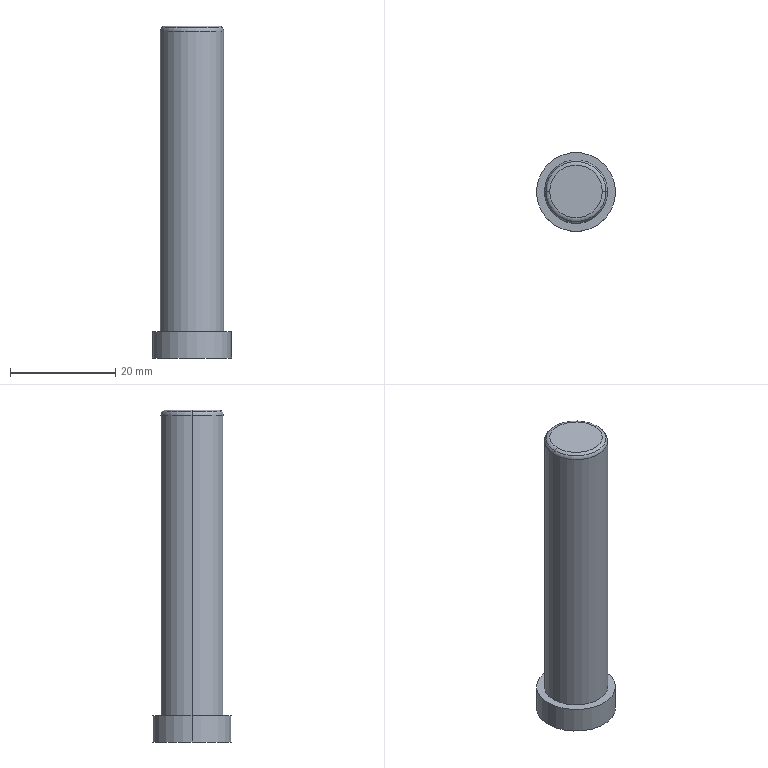Part | STEP file | 1_id1318_x_t | 1 solid | 11 faces | box 15 x 15 x 63 mm | volume 7435 mm3 | cylinder 4 | torus 4 | plane 3 | commonest cylinder face diameters 12 x2 15 x2
STEP:
#1=CARTESIAN_POINT('',(0.,0.,0.));
#2=DIRECTION('',(0.,0.,1.));
#3=DIRECTION('',(1.,0.,0.));
#4=AXIS2_PLACEMENT_3D('',#1,#2,#3);
#5=CARTESIAN_POINT('',(86.275,141.9,-58.));
#6=VERTEX_POINT('',#5);
#7=CARTESIAN_POINT('',(86.275,141.9,-1.));
#8=VERTEX_POINT('',#7);
#9=CARTESIAN_POINT('',(86.275,141.9,-58.));
#10=DIRECTION('',(0.,0.,1.));
#11=VECTOR('',#10,1.);
#12=LINE('',#9,#11);
#13=CARTESIAN_POINT('',(92.275,141.9,-50.));
#14=DIRECTION('',(0.,0.,1.));
#15=DIRECTION('',(1.,0.,0.));
#16=AXIS2_PLACEMENT_3D('',#13,#14,#15);
#17=CYLINDRICAL_SURFACE('',#16,6.);
#18=CARTESIAN_POINT('',(3.142,-8.));
#19=DIRECTION('',(0.,1.));
#20=VECTOR('',#19,1.);
#21=LINE('',#18,#20);
#22=(GEOMETRIC_REPRESENTATION_CONTEXT(2)PARAMETRIC_REPRESENTATION_CONTEXT()REPRESENTATION_CONTEXT('',''));
#23=DEFINITIONAL_REPRESENTATION('',(#21),#22);
#24=PCURVE('',#17,#23);
#25=CARTESIAN_POINT('',(92.275,141.9,-50.));
#26=DIRECTION('',(0.,0.,1.));
#27=DIRECTION('',(1.,0.,0.));
#28=AXIS2_PLACEMENT_3D('',#25,#26,#27);
#29=CYLINDRICAL_SURFACE('',#28,6.);
#30=CARTESIAN_POINT('',(3.142,-8.));
#31=DIRECTION('',(0.,1.));
#32=VECTOR('',#31,1.);
#33=LINE('',#30,#32);
#34=(GEOMETRIC_REPRESENTATION_CONTEXT(2)PARAMETRIC_REPRESENTATION_CONTEXT()REPRESENTATION_CONTEXT('',''));
#35=DEFINITIONAL_REPRESENTATION('',(#33),#34);
#36=PCURVE('',#29,#35);
#37=SURFACE_CURVE('',#12,(#24,#36),.PCURVE_S1.);
#38=EDGE_CURVE('',#6,#8,#37,.T.);
#39=ORIENTED_EDGE('',*,*,#38,.F.);
#40=CARTESIAN_POINT('',(98.275,141.9,-58.));
#41=VERTEX_POINT('',#40);
#42=CARTESIAN_POINT('',(92.275,141.9,-58.));
#43=DIRECTION('',(0.,0.,-1.));
#44=DIRECTION('',(1.,0.,0.));
#45=AXIS2_PLACEMENT_3D('',#42,#43,#44);
#46=CIRCLE('',#45,6.);
#47=CARTESIAN_POINT('',(6.283,-8.));
#48=DIRECTION('',(-1.,0.));
#49=VECTOR('',#48,1.);
#50=LINE('',#47,#49);
#51=(GEOMETRIC_REPRESENTATION_CONTEXT(2)PARAMETRIC_REPRESENTATION_CONTEXT()REPRESENTATION_CONTEXT('',''));
#52=DEFINITIONAL_REPRESENTATION('',(#50),#51);
#53=PCURVE('',#17,#52);
#54=CARTESIAN_POINT('',(92.275,141.9,-58.));
#55=DIRECTION('',(0.,0.,-1.));
#56=DIRECTION('',(-1.,0.,0.));
#57=AXIS2_PLACEMENT_3D('',#54,#55,#56);
#58=PLANE('',#57);
#59=CARTESIAN_POINT('',(0.,0.));
#60=DIRECTION('',(-1.,0.));
#61=AXIS2_PLACEMENT_2D('',#59,#60);
#62=CIRCLE('',#61,6.);
#63=(GEOMETRIC_REPRESENTATION_CONTEXT(2)PARAMETRIC_REPRESENTATION_CONTEXT()REPRESENTATION_CONTEXT('',''));
#64=DEFINITIONAL_REPRESENTATION('',(#62),#63);
#65=PCURVE('',#58,#64);
#66=SURFACE_CURVE('',#46,(#53,#65),.PCURVE_S1.);
#67=EDGE_CURVE('',#41,#6,#66,.T.);
#68=ORIENTED_EDGE('',*,*,#67,.F.);
#69=CARTESIAN_POINT('',(98.275,141.9,-1.));
#70=VERTEX_POINT('',#69);
#71=CARTESIAN_POINT('',(98.275,141.9,-58.));
#72=DIRECTION('',(0.,0.,-1.));
#73=VECTOR('',#72,1.);
#74=LINE('',#71,#73);
#75=CARTESIAN_POINT('',(6.283,-8.));
#76=DIRECTION('',(0.,-1.));
#77=VECTOR('',#76,1.);
#78=LINE('',#75,#77);
#79=(GEOMETRIC_REPRESENTATION_CONTEXT(2)PARAMETRIC_REPRESENTATION_CONTEXT()REPRESENTATION_CONTEXT('',''));
#80=DEFINITIONAL_REPRESENTATION('',(#78),#79);
#81=PCURVE('',#17,#80);
#82=CARTESIAN_POINT('',(0.,-8.));
#83=DIRECTION('',(0.,-1.));
#84=VECTOR('',#83,1.);
#85=LINE('',#82,#84);
#86=(GEOMETRIC_REPRESENTATION_CONTEXT(2)PARAMETRIC_REPRESENTATION_CONTEXT()REPRESENTATION_CONTEXT('',''));
#87=DEFINITIONAL_REPRESENTATION('',(#85),#86);
#88=PCURVE('',#29,#87);
#89=SURFACE_CURVE('',#74,(#81,#88),.PCURVE_S1.);
#90=EDGE_CURVE('',#70,#41,#89,.T.);
#91=ORIENTED_EDGE('',*,*,#90,.F.);
#92=CARTESIAN_POINT('',(92.275,141.9,-1.));
#93=DIRECTION('',(0.,0.,1.));
#94=DIRECTION('',(-1.,0.,0.));
#95=AXIS2_PLACEMENT_3D('',#92,#93,#94);
#96=CIRCLE('',#95,6.);
#97=CARTESIAN_POINT('',(3.142,49.));
#98=DIRECTION('',(1.,0.));
#99=VECTOR('',#98,1.);
#100=LINE('',#97,#99);
#101=(GEOMETRIC_REPRESENTATION_CONTEXT(2)PARAMETRIC_REPRESENTATION_CONTEXT()REPRESENTATION_CONTEXT('',''));
#102=DEFINITIONAL_REPRESENTATION('',(#100),#101);
#103=PCURVE('',#17,#102);
#104=CARTESIAN_POINT('',(92.275,141.9,-1.));
#105=DIRECTION('',(0.,0.,1.));
#106=DIRECTION('',(1.,0.,0.));
#107=AXIS2_PLACEMENT_3D('',#104,#105,#106);
#108=TOROIDAL_SURFACE('',#107,5.,1.);
#109=CARTESIAN_POINT('',(3.142,0.));
#110=DIRECTION('',(1.,0.));
#111=VECTOR('',#110,1.);
#112=LINE('',#109,#111);
#113=(GEOMETRIC_REPRESENTATION_CONTEXT(2)PARAMETRIC_REPRESENTATION_CONTEXT()REPRESENTATION_CONTEXT('',''));
#114=DEFINITIONAL_REPRESENTATION('',(#112),#113);
#115=PCURVE('',#108,#114);
#116=SURFACE_CURVE('',#96,(#103,#115),.PCURVE_S1.);
#117=EDGE_CURVE('',#8,#70,#116,.T.);
#118=ORIENTED_EDGE('',*,*,#117,.F.);
#119=EDGE_LOOP('',(#39,#68,#91,#118));
#120=FACE_BOUND('',#119,.T.);
#121=ADVANCED_FACE('',(#120),#17,.T.);
#122=CARTESIAN_POINT('',(97.982,141.9,-0.2929));
#123=VERTEX_POINT('',#122);
#124=CARTESIAN_POINT('',(97.275,141.9,-1.));
#125=DIRECTION('',(0.,1.,0.));
#126=DIRECTION('',(1.,0.,0.));
#127=AXIS2_PLACEMENT_3D('',#124,#125,#126);
#128=CIRCLE('',#127,1.);
#129=CARTESIAN_POINT('',(6.283,6.283));
#130=DIRECTION('',(0.,-1.));
#131=VECTOR('',#130,1.);
#132=LINE('',#129,#131);
#133=(GEOMETRIC_REPRESENTATION_CONTEXT(2)PARAMETRIC_REPRESENTATION_CONTEXT()REPRESENTATION_CONTEXT('',''));
#134=DEFINITIONAL_REPRESENTATION('',(#132),#133);
#135=PCURVE('',#108,#134);
#136=CARTESIAN_POINT('',(92.275,141.9,-1.));
#137=DIRECTION('',(0.,0.,1.));
#138=DIRECTION('',(1.,0.,0.));
#139=AXIS2_PLACEMENT_3D('',#136,#137,#138);
#140=TOROIDAL_SURFACE('',#139,5.,1.);
#141=CARTESIAN_POINT('',(0.,6.283));
#142=DIRECTION('',(0.,-1.));
#143=VECTOR('',#142,1.);
#144=LINE('',#141,#143);
#145=(GEOMETRIC_REPRESENTATION_CONTEXT(2)PARAMETRIC_REPRESENTATION_CONTEXT()REPRESENTATION_CONTEXT('',''));
#146=DEFINITIONAL_REPRESENTATION('',(#144),#145);
#147=PCURVE('',#140,#146);
#148=SURFACE_CURVE('',#128,(#135,#147),.PCURVE_S1.);
#149=EDGE_CURVE('',#123,#70,#148,.T.);
#150=ORIENTED_EDGE('',*,*,#149,.F.);
#151=CARTESIAN_POINT('',(86.568,141.9,-0.2929));
#152=VERTEX_POINT('',#151);
#153=CARTESIAN_POINT('',(92.275,141.9,-0.2929));
#154=DIRECTION('',(0.,0.,1.));
#155=DIRECTION('',(-1.,0.,0.));
#156=AXIS2_PLACEMENT_3D('',#153,#154,#155);
#157=CIRCLE('',#156,5.707);
#158=CARTESIAN_POINT('',(3.142,0.7854));
#159=DIRECTION('',(1.,0.));
#160=VECTOR('',#159,1.);
#161=LINE('',#158,#160);
#162=(GEOMETRIC_REPRESENTATION_CONTEXT(2)PARAMETRIC_REPRESENTATION_CONTEXT()REPRESENTATION_CONTEXT('',''));
#163=DEFINITIONAL_REPRESENTATION('',(#161),#162);
#164=PCURVE('',#108,#163);
#165=CARTESIAN_POINT('',(92.275,141.9,-1.));
#166=DIRECTION('',(0.,0.,1.));
#167=DIRECTION('',(1.,0.,0.));
#168=AXIS2_PLACEMENT_3D('',#165,#166,#167);
#169=TOROIDAL_SURFACE('',#168,5.,1.);
#170=CARTESIAN_POINT('',(3.142,0.7854));
#171=DIRECTION('',(1.,0.));
#172=VECTOR('',#171,1.);
#173=LINE('',#170,#172);
#174=(GEOMETRIC_REPRESENTATION_CONTEXT(2)PARAMETRIC_REPRESENTATION_CONTEXT()REPRESENTATION_CONTEXT('',''));
#175=DEFINITIONAL_REPRESENTATION('',(#173),#174);
#176=PCURVE('',#169,#175);
#177=SURFACE_CURVE('',#157,(#164,#176),.PCURVE_S1.);
#178=EDGE_CURVE('',#152,#123,#177,.T.);
#179=ORIENTED_EDGE('',*,*,#178,.F.);
#180=CARTESIAN_POINT('',(87.275,141.9,-1.));
#181=DIRECTION('',(0.,1.,0.));
#182=DIRECTION('',(-1.,0.,0.));
#183=AXIS2_PLACEMENT_3D('',#180,#181,#182);
#184=CIRCLE('',#183,1.);
#185=CARTESIAN_POINT('',(3.142,0.));
#186=DIRECTION('',(0.,1.));
#187=VECTOR('',#186,1.);
#188=LINE('',#185,#187);
#189=(GEOMETRIC_REPRESENTATION_CONTEXT(2)PARAMETRIC_REPRESENTATION_CONTEXT()REPRESENTATION_CONTEXT('',''));
#190=DEFINITIONAL_REPRESENTATION('',(#188),#189);
#191=PCURVE('',#108,#190);
#192=CARTESIAN_POINT('',(3.142,0.));
#193=DIRECTION('',(0.,1.));
#194=VECTOR('',#193,1.);
#195=LINE('',#192,#194);
#196=(GEOMETRIC_REPRESENTATION_CONTEXT(2)PARAMETRIC_REPRESENTATION_CONTEXT()REPRESENTATION_CONTEXT('',''));
#197=DEFINITIONAL_REPRESENTATION('',(#195),#196);
#198=PCURVE('',#140,#197);
#199=SURFACE_CURVE('',#184,(#191,#198),.PCURVE_S1.);
#200=EDGE_CURVE('',#8,#152,#199,.T.);
#201=ORIENTED_EDGE('',*,*,#200,.F.);
#202=ORIENTED_EDGE('',*,*,#117,.T.);
#203=EDGE_LOOP('',(#150,#179,#201,#202));
#204=FACE_BOUND('',#203,.T.);
#205=ADVANCED_FACE('',(#204),#108,.T.);
#206=ORIENTED_EDGE('',*,*,#200,.T.);
#207=CARTESIAN_POINT('',(92.275,141.9,-0.2929));
#208=DIRECTION('',(0.,0.,1.));
#209=DIRECTION('',(1.,0.,0.));
#210=AXIS2_PLACEMENT_3D('',#207,#208,#209);
#211=CIRCLE('',#210,5.707);
#212=CARTESIAN_POINT('',(0.,0.7854));
#213=DIRECTION('',(1.,0.));
#214=VECTOR('',#213,1.);
#215=LINE('',#212,#214);
#216=(GEOMETRIC_REPRESENTATION_CONTEXT(2)PARAMETRIC_REPRESENTATION_CONTEXT()REPRESENTATION_CONTEXT('',''));
#217=DEFINITIONAL_REPRESENTATION('',(#215),#216);
#218=PCURVE('',#140,#217);
#219=CARTESIAN_POINT('',(92.275,141.9,-1.));
#220=DIRECTION('',(0.,0.,1.));
#221=DIRECTION('',(1.,0.,0.));
#222=AXIS2_PLACEMENT_3D('',#219,#220,#221);
#223=TOROIDAL_SURFACE('',#222,5.,1.);
#224=CARTESIAN_POINT('',(0.,0.7854));
#225=DIRECTION('',(1.,0.));
#226=VECTOR('',#225,1.);
#227=LINE('',#224,#226);
#228=(GEOMETRIC_REPRESENTATION_CONTEXT(2)PARAMETRIC_REPRESENTATION_CONTEXT()REPRESENTATION_CONTEXT('',''));
#229=DEFINITIONAL_REPRESENTATION('',(#227),#228);
#230=PCURVE('',#223,#229);
#231=SURFACE_CURVE('',#211,(#218,#230),.PCURVE_S1.);
#232=EDGE_CURVE('',#123,#152,#231,.T.);
#233=ORIENTED_EDGE('',*,*,#232,.F.);
#234=ORIENTED_EDGE('',*,*,#149,.T.);
#235=CARTESIAN_POINT('',(92.275,141.9,-1.));
#236=DIRECTION('',(0.,0.,1.));
#237=DIRECTION('',(1.,0.,0.));
#238=AXIS2_PLACEMENT_3D('',#235,#236,#237);
#239=CIRCLE('',#238,6.);
#240=CARTESIAN_POINT('',(0.,0.));
#241=DIRECTION('',(1.,0.));
#242=VECTOR('',#241,1.);
#243=LINE('',#240,#242);
#244=(GEOMETRIC_REPRESENTATION_CONTEXT(2)PARAMETRIC_REPRESENTATION_CONTEXT()REPRESENTATION_CONTEXT('',''));
#245=DEFINITIONAL_REPRESENTATION('',(#243),#244);
#246=PCURVE('',#140,#245);
#247=CARTESIAN_POINT('',(0.,49.));
#248=DIRECTION('',(1.,0.));
#249=VECTOR('',#248,1.);
#250=LINE('',#247,#249);
#251=(GEOMETRIC_REPRESENTATION_CONTEXT(2)PARAMETRIC_REPRESENTATION_CONTEXT()REPRESENTATION_CONTEXT('',''));
#252=DEFINITIONAL_REPRESENTATION('',(#250),#251);
#253=PCURVE('',#29,#252);
#254=SURFACE_CURVE('',#239,(#246,#253),.PCURVE_S1.);
#255=EDGE_CURVE('',#70,#8,#254,.T.);
#256=ORIENTED_EDGE('',*,*,#255,.T.);
#257=EDGE_LOOP('',(#206,#233,#234,#256));
#258=FACE_BOUND('',#257,.T.);
#259=ADVANCED_FACE('',(#258),#140,.T.);
#260=ORIENTED_EDGE('',*,*,#90,.T.);
#261=CARTESIAN_POINT('',(92.275,141.9,-58.));
#262=DIRECTION('',(0.,0.,-1.));
#263=DIRECTION('',(-1.,0.,0.));
#264=AXIS2_PLACEMENT_3D('',#261,#262,#263);
#265=CIRCLE('',#264,6.);
#266=CARTESIAN_POINT('',(3.142,-8.));
#267=DIRECTION('',(-1.,0.));
#268=VECTOR('',#267,1.);
#269=LINE('',#266,#268);
#270=(GEOMETRIC_REPRESENTATION_CONTEXT(2)PARAMETRIC_REPRESENTATION_CONTEXT()REPRESENTATION_CONTEXT('',''));
#271=DEFINITIONAL_REPRESENTATION('',(#269),#270);
#272=PCURVE('',#29,#271);
#273=CARTESIAN_POINT('',(0.,0.));
#274=DIRECTION('',(1.,0.));
#275=AXIS2_PLACEMENT_2D('',#273,#274);
#276=CIRCLE('',#275,6.);
#277=(GEOMETRIC_REPRESENTATION_CONTEXT(2)PARAMETRIC_REPRESENTATION_CONTEXT()REPRESENTATION_CONTEXT('',''));
#278=DEFINITIONAL_REPRESENTATION('',(#276),#277);
#279=PCURVE('',#58,#278);
#280=SURFACE_CURVE('',#265,(#272,#279),.PCURVE_S1.);
#281=EDGE_CURVE('',#6,#41,#280,.T.);
#282=ORIENTED_EDGE('',*,*,#281,.F.);
#283=ORIENTED_EDGE('',*,*,#38,.T.);
#284=ORIENTED_EDGE('',*,*,#255,.F.);
#285=EDGE_LOOP('',(#260,#282,#283,#284));
#286=FACE_BOUND('',#285,.T.);
#287=ADVANCED_FACE('',(#286),#29,.T.);
#288=CARTESIAN_POINT('',(84.775,141.9,-58.));
#289=VERTEX_POINT('',#288);
#290=CARTESIAN_POINT('',(99.775,141.9,-58.));
#291=VERTEX_POINT('',#290);
#292=CARTESIAN_POINT('',(92.275,141.9,-58.));
#293=DIRECTION('',(0.,0.,1.));
#294=DIRECTION('',(-1.,0.,0.));
#295=AXIS2_PLACEMENT_3D('',#292,#293,#294);
#296=CIRCLE('',#295,7.5);
#297=CARTESIAN_POINT('',(7.5,0.));
#298=CARTESIAN_POINT('',(7.5,-12.99));
#299=CARTESIAN_POINT('',(-3.75,-6.495));
#300=CARTESIAN_POINT('',(-15.,0.));
#301=CARTESIAN_POINT('',(-3.75,6.495));
#302=CARTESIAN_POINT('',(7.5,12.99));
#303=CARTESIAN_POINT('',(7.5,0.));
#304=(BOUNDED_CURVE()B_SPLINE_CURVE(2,(#297,#298,#299,#300,#301,#302,#303),.UNSPECIFIED.,.T.,.F.)B_SPLINE_CURVE_WITH_KNOTS((1,2,2,2,2,1),(-2.094,0.,2.094,4.189,6.283,8.378),.UNSPECIFIED.)CURVE()GEOMETRIC_REPRESENTATION_ITEM()RATIONAL_B_SPLINE_CURVE((1.,0.5,1.,0.5,1.,0.5,1.))REPRESENTATION_ITEM(''));
#305=(GEOMETRIC_REPRESENTATION_CONTEXT(2)PARAMETRIC_REPRESENTATION_CONTEXT()REPRESENTATION_CONTEXT('',''));
#306=DEFINITIONAL_REPRESENTATION('',(#304),#305);
#307=PCURVE('',#58,#306);
#308=CARTESIAN_POINT('',(92.275,141.9,-58.));
#309=DIRECTION('',(0.,0.,-1.));
#310=DIRECTION('',(-1.,0.,0.));
#311=AXIS2_PLACEMENT_3D('',#308,#309,#310);
#312=CYLINDRICAL_SURFACE('',#311,7.5);
#313=CARTESIAN_POINT('',(6.283,0.));
#314=DIRECTION('',(-1.,0.));
#315=VECTOR('',#314,1.);
#316=LINE('',#313,#315);
#317=(GEOMETRIC_REPRESENTATION_CONTEXT(2)PARAMETRIC_REPRESENTATION_CONTEXT()REPRESENTATION_CONTEXT('',''));
#318=DEFINITIONAL_REPRESENTATION('',(#316),#317);
#319=PCURVE('',#312,#318);
#320=SURFACE_CURVE('',#296,(#307,#319),.PCURVE_S1.);
#321=EDGE_CURVE('',#289,#291,#320,.T.);
#322=ORIENTED_EDGE('',*,*,#321,.T.);
#323=CARTESIAN_POINT('',(92.275,141.9,-58.));
#324=DIRECTION('',(0.,0.,1.));
#325=DIRECTION('',(1.,0.,0.));
#326=AXIS2_PLACEMENT_3D('',#323,#324,#325);
#327=CIRCLE('',#326,7.5);
#328=CARTESIAN_POINT('',(-7.5,0.));
#329=CARTESIAN_POINT('',(-7.5,12.99));
#330=CARTESIAN_POINT('',(3.75,6.495));
#331=CARTESIAN_POINT('',(15.,0.));
#332=CARTESIAN_POINT('',(3.75,-6.495));
#333=CARTESIAN_POINT('',(-7.5,-12.99));
#334=CARTESIAN_POINT('',(-7.5,0.));
#335=(BOUNDED_CURVE()B_SPLINE_CURVE(2,(#328,#329,#330,#331,#332,#333,#334),.UNSPECIFIED.,.T.,.F.)B_SPLINE_CURVE_WITH_KNOTS((1,2,2,2,2,1),(-2.094,0.,2.094,4.189,6.283,8.378),.UNSPECIFIED.)CURVE()GEOMETRIC_REPRESENTATION_ITEM()RATIONAL_B_SPLINE_CURVE((1.,0.5,1.,0.5,1.,0.5,1.))REPRESENTATION_ITEM(''));
#336=(GEOMETRIC_REPRESENTATION_CONTEXT(2)PARAMETRIC_REPRESENTATION_CONTEXT()REPRESENTATION_CONTEXT('',''));
#337=DEFINITIONAL_REPRESENTATION('',(#335),#336);
#338=PCURVE('',#58,#337);
#339=CARTESIAN_POINT('',(92.275,141.9,-58.));
#340=DIRECTION('',(0.,0.,-1.));
#341=DIRECTION('',(-1.,0.,0.));
#342=AXIS2_PLACEMENT_3D('',#339,#340,#341);
#343=CYLINDRICAL_SURFACE('',#342,7.5);
#344=CARTESIAN_POINT('',(3.142,0.));
#345=DIRECTION('',(-1.,0.));
#346=VECTOR('',#345,1.);
#347=LINE('',#344,#346);
#348=(GEOMETRIC_REPRESENTATION_CONTEXT(2)PARAMETRIC_REPRESENTATION_CONTEXT()REPRESENTATION_CONTEXT('',''));
#349=DEFINITIONAL_REPRESENTATION('',(#347),#348);
#350=PCURVE('',#343,#349);
#351=SURFACE_CURVE('',#327,(#338,#350),.PCURVE_S1.);
#352=EDGE_CURVE('',#291,#289,#351,.T.);
#353=ORIENTED_EDGE('',*,*,#352,.T.);
#354=EDGE_LOOP('',(#322,#353));
#355=FACE_BOUND('',#354,.T.);
#356=ORIENTED_EDGE('',*,*,#67,.T.);
#357=ORIENTED_EDGE('',*,*,#281,.T.);
#358=EDGE_LOOP('',(#356,#357));
#359=FACE_BOUND('',#358,.T.);
#360=ADVANCED_FACE('',(#355,#359),#58,.F.);
#361=CARTESIAN_POINT('',(99.775,141.9,-63.));
#362=VERTEX_POINT('',#361);
#363=CARTESIAN_POINT('',(99.775,141.9,-58.));
#364=DIRECTION('',(0.,0.,-1.));
#365=VECTOR('',#364,1.);
#366=LINE('',#363,#365);
#367=CARTESIAN_POINT('',(3.142,0.));
#368=DIRECTION('',(0.,1.));
#369=VECTOR('',#368,1.);
#370=LINE('',#367,#369);
#371=(GEOMETRIC_REPRESENTATION_CONTEXT(2)PARAMETRIC_REPRESENTATION_CONTEXT()REPRESENTATION_CONTEXT('',''));
#372=DEFINITIONAL_REPRESENTATION('',(#370),#371);
#373=PCURVE('',#343,#372);
#374=CARTESIAN_POINT('',(3.142,0.));
#375=DIRECTION('',(0.,1.));
#376=VECTOR('',#375,1.);
#377=LINE('',#374,#376);
#378=(GEOMETRIC_REPRESENTATION_CONTEXT(2)PARAMETRIC_REPRESENTATION_CONTEXT()REPRESENTATION_CONTEXT('',''));
#379=DEFINITIONAL_REPRESENTATION('',(#377),#378);
#380=PCURVE('',#312,#379);
#381=SURFACE_CURVE('',#366,(#373,#380),.PCURVE_S1.);
#382=EDGE_CURVE('',#291,#362,#381,.T.);
#383=ORIENTED_EDGE('',*,*,#382,.T.);
#384=CARTESIAN_POINT('',(84.775,141.9,-63.));
#385=VERTEX_POINT('',#384);
#386=CARTESIAN_POINT('',(92.275,141.9,-63.));
#387=DIRECTION('',(0.,0.,-1.));
#388=DIRECTION('',(-1.,0.,0.));
#389=AXIS2_PLACEMENT_3D('',#386,#387,#388);
#390=CIRCLE('',#389,7.5);
#391=CARTESIAN_POINT('',(0.,5.));
#392=DIRECTION('',(1.,0.));
#393=VECTOR('',#392,1.);
#394=LINE('',#391,#393);
#395=(GEOMETRIC_REPRESENTATION_CONTEXT(2)PARAMETRIC_REPRESENTATION_CONTEXT()REPRESENTATION_CONTEXT('',''));
#396=DEFINITIONAL_REPRESENTATION('',(#394),#395);
#397=PCURVE('',#343,#396);
#398=CARTESIAN_POINT('',(92.275,141.9,-63.));
#399=DIRECTION('',(0.,0.,-1.));
#400=DIRECTION('',(-1.,0.,0.));
#401=AXIS2_PLACEMENT_3D('',#398,#399,#400);
#402=PLANE('',#401);
#403=CARTESIAN_POINT('',(0.,0.));
#404=DIRECTION('',(1.,0.));
#405=AXIS2_PLACEMENT_2D('',#403,#404);
#406=CIRCLE('',#405,7.5);
#407=(GEOMETRIC_REPRESENTATION_CONTEXT(2)PARAMETRIC_REPRESENTATION_CONTEXT()REPRESENTATION_CONTEXT('',''));
#408=DEFINITIONAL_REPRESENTATION('',(#406),#407);
#409=PCURVE('',#402,#408);
#410=SURFACE_CURVE('',#390,(#397,#409),.PCURVE_S1.);
#411=EDGE_CURVE('',#385,#362,#410,.T.);
#412=ORIENTED_EDGE('',*,*,#411,.F.);
#413=CARTESIAN_POINT('',(84.775,141.9,-58.));
#414=DIRECTION('',(0.,0.,1.));
#415=VECTOR('',#414,1.);
#416=LINE('',#413,#415);
#417=CARTESIAN_POINT('',(0.,0.));
#418=DIRECTION('',(0.,-1.));
#419=VECTOR('',#418,1.);
#420=LINE('',#417,#419);
#421=(GEOMETRIC_REPRESENTATION_CONTEXT(2)PARAMETRIC_REPRESENTATION_CONTEXT()REPRESENTATION_CONTEXT('',''));
#422=DEFINITIONAL_REPRESENTATION('',(#420),#421);
#423=PCURVE('',#343,#422);
#424=CARTESIAN_POINT('',(6.283,0.));
#425=DIRECTION('',(0.,-1.));
#426=VECTOR('',#425,1.);
#427=LINE('',#424,#426);
#428=(GEOMETRIC_REPRESENTATION_CONTEXT(2)PARAMETRIC_REPRESENTATION_CONTEXT()REPRESENTATION_CONTEXT('',''));
#429=DEFINITIONAL_REPRESENTATION('',(#427),#428);
#430=PCURVE('',#312,#429);
#431=SURFACE_CURVE('',#416,(#423,#430),.PCURVE_S1.);
#432=EDGE_CURVE('',#385,#289,#431,.T.);
#433=ORIENTED_EDGE('',*,*,#432,.T.);
#434=ORIENTED_EDGE('',*,*,#352,.F.);
#435=EDGE_LOOP('',(#383,#412,#433,#434));
#436=FACE_BOUND('',#435,.T.);
#437=ADVANCED_FACE('',(#436),#343,.T.);
#438=ORIENTED_EDGE('',*,*,#432,.F.);
#439=CARTESIAN_POINT('',(92.275,141.9,-63.));
#440=DIRECTION('',(0.,0.,-1.));
#441=DIRECTION('',(1.,0.,0.));
#442=AXIS2_PLACEMENT_3D('',#439,#440,#441);
#443=CIRCLE('',#442,7.5);
#444=CARTESIAN_POINT('',(3.142,5.));
#445=DIRECTION('',(1.,0.));
#446=VECTOR('',#445,1.);
#447=LINE('',#444,#446);
#448=(GEOMETRIC_REPRESENTATION_CONTEXT(2)PARAMETRIC_REPRESENTATION_CONTEXT()REPRESENTATION_CONTEXT('',''));
#449=DEFINITIONAL_REPRESENTATION('',(#447),#448);
#450=PCURVE('',#312,#449);
#451=CARTESIAN_POINT('',(0.,0.));
#452=DIRECTION('',(-1.,0.));
#453=AXIS2_PLACEMENT_2D('',#451,#452);
#454=CIRCLE('',#453,7.5);
#455=(GEOMETRIC_REPRESENTATION_CONTEXT(2)PARAMETRIC_REPRESENTATION_CONTEXT()REPRESENTATION_CONTEXT('',''));
#456=DEFINITIONAL_REPRESENTATION('',(#454),#455);
#457=PCURVE('',#402,#456);
#458=SURFACE_CURVE('',#443,(#450,#457),.PCURVE_S1.);
#459=EDGE_CURVE('',#362,#385,#458,.T.);
#460=ORIENTED_EDGE('',*,*,#459,.F.);
#461=ORIENTED_EDGE('',*,*,#382,.F.);
#462=ORIENTED_EDGE('',*,*,#321,.F.);
#463=EDGE_LOOP('',(#438,#460,#461,#462));
#464=FACE_BOUND('',#463,.T.);
#465=ADVANCED_FACE('',(#464),#312,.T.);
#466=ORIENTED_EDGE('',*,*,#411,.T.);
#467=ORIENTED_EDGE('',*,*,#459,.T.);
#468=EDGE_LOOP('',(#466,#467));
#469=FACE_BOUND('',#468,.T.);
#470=ADVANCED_FACE('',(#469),#402,.T.);
#471=CARTESIAN_POINT('',(97.275,141.9,-0.00002908));
#472=VERTEX_POINT('',#471);
#473=CARTESIAN_POINT('',(97.275,141.9,-1.));
#474=DIRECTION('',(0.,-1.,0.));
#475=DIRECTION('',(0.7071,0.,0.7071));
#476=AXIS2_PLACEMENT_3D('',#473,#474,#475);
#477=CIRCLE('',#476,1.);
#478=CARTESIAN_POINT('',(0.,0.7854));
#479=DIRECTION('',(0.,1.));
#480=VECTOR('',#479,1.);
#481=LINE('',#478,#480);
#482=(GEOMETRIC_REPRESENTATION_CONTEXT(2)PARAMETRIC_REPRESENTATION_CONTEXT()REPRESENTATION_CONTEXT('',''));
#483=DEFINITIONAL_REPRESENTATION('',(#481),#482);
#484=PCURVE('',#223,#483);
#485=CARTESIAN_POINT('',(6.283,0.7854));
#486=DIRECTION('',(0.,1.));
#487=VECTOR('',#486,1.);
#488=LINE('',#485,#487);
#489=(GEOMETRIC_REPRESENTATION_CONTEXT(2)PARAMETRIC_REPRESENTATION_CONTEXT()REPRESENTATION_CONTEXT('',''));
#490=DEFINITIONAL_REPRESENTATION('',(#488),#489);
#491=PCURVE('',#169,#490);
#492=SURFACE_CURVE('',#477,(#484,#491),.PCURVE_S1.);
#493=EDGE_CURVE('',#123,#472,#492,.T.);
#494=ORIENTED_EDGE('',*,*,#493,.F.);
#495=ORIENTED_EDGE('',*,*,#232,.T.);
#496=CARTESIAN_POINT('',(87.275,141.9,-0.00002908));
#497=VERTEX_POINT('',#496);
#498=CARTESIAN_POINT('',(87.275,141.9,-1.));
#499=DIRECTION('',(0.,-1.,0.));
#500=DIRECTION('',(-0.7071,0.,0.7071));
#501=AXIS2_PLACEMENT_3D('',#498,#499,#500);
#502=CIRCLE('',#501,1.);
#503=CARTESIAN_POINT('',(3.142,7.069));
#504=DIRECTION('',(0.,-1.));
#505=VECTOR('',#504,1.);
#506=LINE('',#503,#505);
#507=(GEOMETRIC_REPRESENTATION_CONTEXT(2)PARAMETRIC_REPRESENTATION_CONTEXT()REPRESENTATION_CONTEXT('',''));
#508=DEFINITIONAL_REPRESENTATION('',(#506),#507);
#509=PCURVE('',#223,#508);
#510=CARTESIAN_POINT('',(3.142,7.069));
#511=DIRECTION('',(0.,-1.));
#512=VECTOR('',#511,1.);
#513=LINE('',#510,#512);
#514=(GEOMETRIC_REPRESENTATION_CONTEXT(2)PARAMETRIC_REPRESENTATION_CONTEXT()REPRESENTATION_CONTEXT('',''));
#515=DEFINITIONAL_REPRESENTATION('',(#513),#514);
#516=PCURVE('',#169,#515);
#517=SURFACE_CURVE('',#502,(#509,#516),.PCURVE_S1.);
#518=EDGE_CURVE('',#497,#152,#517,.T.);
#519=ORIENTED_EDGE('',*,*,#518,.F.);
#520=CARTESIAN_POINT('',(92.275,141.9,-0.00002908));
#521=DIRECTION('',(0.,0.,1.));
#522=DIRECTION('',(1.,0.,0.));
#523=AXIS2_PLACEMENT_3D('',#520,#521,#522);
#524=CIRCLE('',#523,5.);
#525=CARTESIAN_POINT('',(0.,1.571));
#526=DIRECTION('',(1.,0.));
#527=VECTOR('',#526,1.);
#528=LINE('',#525,#527);
#529=(GEOMETRIC_REPRESENTATION_CONTEXT(2)PARAMETRIC_REPRESENTATION_CONTEXT()REPRESENTATION_CONTEXT('',''));
#530=DEFINITIONAL_REPRESENTATION('',(#528),#529);
#531=PCURVE('',#223,#530);
#532=CARTESIAN_POINT('',(92.275,141.9,-0.00002908));
#533=DIRECTION('',(0.,0.,1.));
#534=DIRECTION('',(1.,0.,0.));
#535=AXIS2_PLACEMENT_3D('',#532,#533,#534);
#536=PLANE('',#535);
#537=CARTESIAN_POINT('',(0.,0.));
#538=DIRECTION('',(1.,0.));
#539=AXIS2_PLACEMENT_2D('',#537,#538);
#540=CIRCLE('',#539,5.);
#541=(GEOMETRIC_REPRESENTATION_CONTEXT(2)PARAMETRIC_REPRESENTATION_CONTEXT()REPRESENTATION_CONTEXT('',''));
#542=DEFINITIONAL_REPRESENTATION('',(#540),#541);
#543=PCURVE('',#536,#542);
#544=SURFACE_CURVE('',#524,(#531,#543),.PCURVE_S1.);
#545=EDGE_CURVE('',#472,#497,#544,.T.);
#546=ORIENTED_EDGE('',*,*,#545,.F.);
#547=EDGE_LOOP('',(#494,#495,#519,#546));
#548=FACE_BOUND('',#547,.T.);
#549=ADVANCED_FACE('',(#548),#223,.T.);
#550=ORIENTED_EDGE('',*,*,#545,.T.);
#551=CARTESIAN_POINT('',(92.275,141.9,-0.00002908));
#552=DIRECTION('',(0.,0.,1.));
#553=DIRECTION('',(-1.,0.,0.));
#554=AXIS2_PLACEMENT_3D('',#551,#552,#553);
#555=CIRCLE('',#554,5.);
#556=CARTESIAN_POINT('',(0.,0.));
#557=DIRECTION('',(-1.,0.));
#558=AXIS2_PLACEMENT_2D('',#556,#557);
#559=CIRCLE('',#558,5.);
#560=(GEOMETRIC_REPRESENTATION_CONTEXT(2)PARAMETRIC_REPRESENTATION_CONTEXT()REPRESENTATION_CONTEXT('',''));
#561=DEFINITIONAL_REPRESENTATION('',(#559),#560);
#562=PCURVE('',#536,#561);
#563=CARTESIAN_POINT('',(3.142,1.571));
#564=DIRECTION('',(1.,0.));
#565=VECTOR('',#564,1.);
#566=LINE('',#563,#565);
#567=(GEOMETRIC_REPRESENTATION_CONTEXT(2)PARAMETRIC_REPRESENTATION_CONTEXT()REPRESENTATION_CONTEXT('',''));
#568=DEFINITIONAL_REPRESENTATION('',(#566),#567);
#569=PCURVE('',#169,#568);
#570=SURFACE_CURVE('',#555,(#562,#569),.PCURVE_S1.);
#571=EDGE_CURVE('',#497,#472,#570,.T.);
#572=ORIENTED_EDGE('',*,*,#571,.T.);
#573=EDGE_LOOP('',(#550,#572));
#574=FACE_BOUND('',#573,.T.);
#575=ADVANCED_FACE('',(#574),#536,.T.);
#576=ORIENTED_EDGE('',*,*,#518,.T.);
#577=ORIENTED_EDGE('',*,*,#178,.T.);
#578=ORIENTED_EDGE('',*,*,#493,.T.);
#579=ORIENTED_EDGE('',*,*,#571,.F.);
#580=EDGE_LOOP('',(#576,#577,#578,#579));
#581=FACE_BOUND('',#580,.T.);
#582=ADVANCED_FACE('',(#581),#169,.T.);
#583=CLOSED_SHELL('',(#121,#205,#259,#287,#360,#437,#465,#470,#549,#575,#582));
#584=MANIFOLD_SOLID_BREP('',#583);
#585=(LENGTH_UNIT()NAMED_UNIT(*)SI_UNIT(.MILLI.,.METRE.));
#586=UNCERTAINTY_MEASURE_WITH_UNIT(LENGTH_MEASURE(0.0000001),#585,'','');
#587=(NAMED_UNIT(*)PLANE_ANGLE_UNIT()SI_UNIT($,.RADIAN.));
#588=(NAMED_UNIT(*)SI_UNIT($,.STERADIAN.)SOLID_ANGLE_UNIT());
#589=(GEOMETRIC_REPRESENTATION_CONTEXT(3)GLOBAL_UNCERTAINTY_ASSIGNED_CONTEXT((#586))GLOBAL_UNIT_ASSIGNED_CONTEXT((#585,#587,#588))REPRESENTATION_CONTEXT('',''));
#590=ADVANCED_BREP_SHAPE_REPRESENTATION('',(#4,#584),#589);